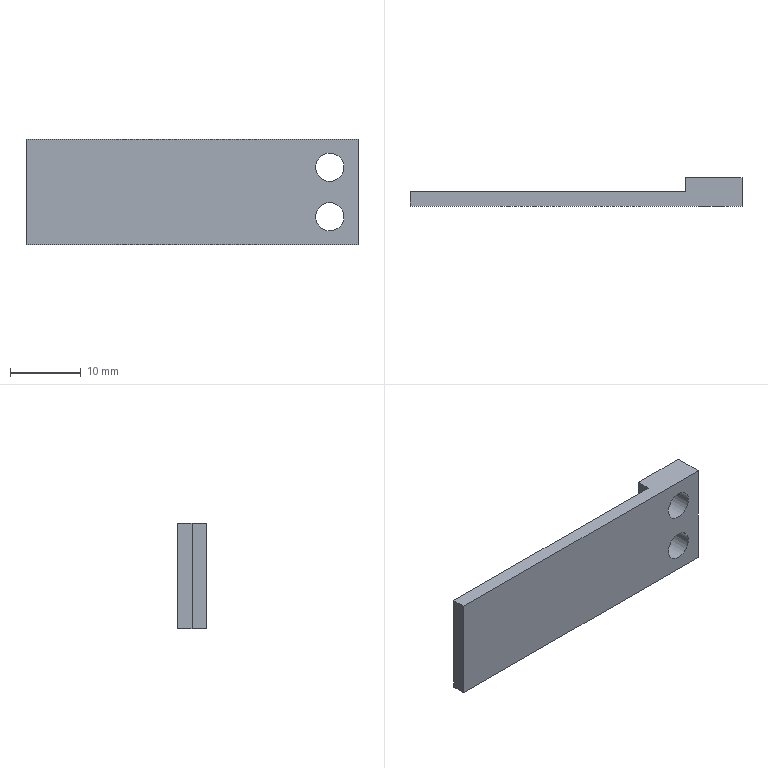Part | SolidWorks | features Extrusion 1, ICE 1 | 1 solid | 12 faces | box 47 x 4 x 15 mm | volume 1549 mm3 | plane 8 | cylinder 4 | commonest cylinder face diameters 4 x4
STEP:
#1=CARTESIAN_POINT('',(41.,0.,-3.5));
#2=VERTEX_POINT('',#1);
#3=CARTESIAN_POINT('',(45.,0.,-3.5));
#4=VERTEX_POINT('',#3);
#5=CARTESIAN_POINT('',(43.,0.,-3.5));
#6=DIRECTION('',(0.,-1.,0.));
#7=DIRECTION('',(0.,0.,1.));
#8=AXIS2_PLACEMENT_3D('',#5,#6,#7);
#9=CIRCLE('',#8,2.);
#10=EDGE_CURVE('',#2,#4,#9,.T.);
#11=ORIENTED_EDGE('',*,*,#10,.T.);
#12=CARTESIAN_POINT('',(45.,4.,-3.5));
#13=VERTEX_POINT('',#12);
#14=CARTESIAN_POINT('',(45.,-0.001,-3.5));
#15=DIRECTION('',(0.,1.,0.));
#16=VECTOR('',#15,1000.);
#17=LINE('',#14,#16);
#18=EDGE_CURVE('',#4,#13,#17,.T.);
#19=ORIENTED_EDGE('',*,*,#18,.T.);
#20=CARTESIAN_POINT('',(41.,4.,-3.5));
#21=VERTEX_POINT('',#20);
#22=CARTESIAN_POINT('',(43.,4.,-3.5));
#23=DIRECTION('',(0.,1.,0.));
#24=DIRECTION('',(-1.,0.,0.));
#25=AXIS2_PLACEMENT_3D('',#22,#23,#24);
#26=CIRCLE('',#25,2.);
#27=EDGE_CURVE('',#13,#21,#26,.T.);
#28=ORIENTED_EDGE('',*,*,#27,.T.);
#29=CARTESIAN_POINT('',(41.,-0.001,-3.5));
#30=DIRECTION('',(0.,1.,0.));
#31=VECTOR('',#30,1000.);
#32=LINE('',#29,#31);
#33=EDGE_CURVE('',#2,#21,#32,.T.);
#34=ORIENTED_EDGE('',*,*,#33,.F.);
#35=EDGE_LOOP('',(#11,#19,#28,#34));
#36=FACE_OUTER_BOUND('',#35,.T.);
#37=CARTESIAN_POINT('',(43.,-0.001,-3.5));
#38=DIRECTION('',(0.,1.,0.));
#39=DIRECTION('',(-1.,0.,0.));
#40=AXIS2_PLACEMENT_3D('',#37,#38,#39);
#41=CYLINDRICAL_SURFACE('',#40,2.);
#42=ADVANCED_FACE('',(#36),#41,.F.);
#43=CARTESIAN_POINT('',(41.,0.,3.5));
#44=VERTEX_POINT('',#43);
#45=CARTESIAN_POINT('',(45.,0.,3.5));
#46=VERTEX_POINT('',#45);
#47=CARTESIAN_POINT('',(43.,0.,3.5));
#48=DIRECTION('',(0.,-1.,0.));
#49=DIRECTION('',(0.,0.,1.));
#50=AXIS2_PLACEMENT_3D('',#47,#48,#49);
#51=CIRCLE('',#50,2.);
#52=EDGE_CURVE('',#44,#46,#51,.T.);
#53=ORIENTED_EDGE('',*,*,#52,.T.);
#54=CARTESIAN_POINT('',(45.,4.,3.5));
#55=VERTEX_POINT('',#54);
#56=CARTESIAN_POINT('',(45.,-0.001,3.5));
#57=DIRECTION('',(0.,1.,0.));
#58=VECTOR('',#57,1000.);
#59=LINE('',#56,#58);
#60=EDGE_CURVE('',#46,#55,#59,.T.);
#61=ORIENTED_EDGE('',*,*,#60,.T.);
#62=CARTESIAN_POINT('',(41.,4.,3.5));
#63=VERTEX_POINT('',#62);
#64=CARTESIAN_POINT('',(43.,4.,3.5));
#65=DIRECTION('',(0.,1.,0.));
#66=DIRECTION('',(-1.,0.,0.));
#67=AXIS2_PLACEMENT_3D('',#64,#65,#66);
#68=CIRCLE('',#67,2.);
#69=EDGE_CURVE('',#55,#63,#68,.T.);
#70=ORIENTED_EDGE('',*,*,#69,.T.);
#71=CARTESIAN_POINT('',(41.,-0.001,3.5));
#72=DIRECTION('',(0.,1.,0.));
#73=VECTOR('',#72,1000.);
#74=LINE('',#71,#73);
#75=EDGE_CURVE('',#44,#63,#74,.T.);
#76=ORIENTED_EDGE('',*,*,#75,.F.);
#77=EDGE_LOOP('',(#53,#61,#70,#76));
#78=FACE_OUTER_BOUND('',#77,.T.);
#79=CARTESIAN_POINT('',(43.,-0.001,3.5));
#80=DIRECTION('',(0.,1.,0.));
#81=DIRECTION('',(-1.,0.,0.));
#82=AXIS2_PLACEMENT_3D('',#79,#80,#81);
#83=CYLINDRICAL_SURFACE('',#82,2.);
#84=ADVANCED_FACE('',(#78),#83,.F.);
#85=CARTESIAN_POINT('',(0.,2.,-7.5));
#86=VERTEX_POINT('',#85);
#87=CARTESIAN_POINT('',(0.,0.,-7.5));
#88=VERTEX_POINT('',#87);
#89=CARTESIAN_POINT('',(0.,2.,-7.5));
#90=DIRECTION('',(0.,-1.,0.));
#91=VECTOR('',#90,1000.);
#92=LINE('',#89,#91);
#93=EDGE_CURVE('',#86,#88,#92,.T.);
#94=ORIENTED_EDGE('',*,*,#93,.T.);
#95=CARTESIAN_POINT('',(0.,0.,7.5));
#96=VERTEX_POINT('',#95);
#97=CARTESIAN_POINT('',(0.,0.,7.5));
#98=DIRECTION('',(0.,0.,-1.));
#99=VECTOR('',#98,1000.);
#100=LINE('',#97,#99);
#101=EDGE_CURVE('',#96,#88,#100,.T.);
#102=ORIENTED_EDGE('',*,*,#101,.F.);
#103=CARTESIAN_POINT('',(0.,2.,7.5));
#104=VERTEX_POINT('',#103);
#105=CARTESIAN_POINT('',(0.,2.,7.5));
#106=DIRECTION('',(0.,-1.,0.));
#107=VECTOR('',#106,1000.);
#108=LINE('',#105,#107);
#109=EDGE_CURVE('',#104,#96,#108,.T.);
#110=ORIENTED_EDGE('',*,*,#109,.F.);
#111=CARTESIAN_POINT('',(0.,2.,7.5));
#112=DIRECTION('',(0.,0.,-1.));
#113=VECTOR('',#112,1000.);
#114=LINE('',#111,#113);
#115=EDGE_CURVE('',#104,#86,#114,.T.);
#116=ORIENTED_EDGE('',*,*,#115,.T.);
#117=EDGE_LOOP('',(#94,#102,#110,#116));
#118=FACE_OUTER_BOUND('',#117,.T.);
#119=CARTESIAN_POINT('',(0.,2.,7.5));
#120=DIRECTION('',(1.,0.,0.));
#121=DIRECTION('',(0.,0.,-1.));
#122=AXIS2_PLACEMENT_3D('',#119,#120,#121);
#123=PLANE('',#122);
#124=ADVANCED_FACE('',(#118),#123,.F.);
#125=ORIENTED_EDGE('',*,*,#10,.F.);
#126=CARTESIAN_POINT('',(43.,0.,-3.5));
#127=DIRECTION('',(0.,-1.,0.));
#128=DIRECTION('',(0.,0.,1.));
#129=AXIS2_PLACEMENT_3D('',#126,#127,#128);
#130=CIRCLE('',#129,2.);
#131=EDGE_CURVE('',#4,#2,#130,.T.);
#132=ORIENTED_EDGE('',*,*,#131,.F.);
#133=EDGE_LOOP('',(#125,#132));
#134=FACE_BOUND('',#133,.T.);
#135=ORIENTED_EDGE('',*,*,#52,.F.);
#136=CARTESIAN_POINT('',(43.,0.,3.5));
#137=DIRECTION('',(0.,-1.,0.));
#138=DIRECTION('',(0.,0.,1.));
#139=AXIS2_PLACEMENT_3D('',#136,#137,#138);
#140=CIRCLE('',#139,2.);
#141=EDGE_CURVE('',#46,#44,#140,.T.);
#142=ORIENTED_EDGE('',*,*,#141,.F.);
#143=EDGE_LOOP('',(#135,#142));
#144=FACE_BOUND('',#143,.T.);
#145=CARTESIAN_POINT('',(47.,0.,-7.5));
#146=VERTEX_POINT('',#145);
#147=CARTESIAN_POINT('',(0.,0.,-7.5));
#148=DIRECTION('',(1.,0.,0.));
#149=VECTOR('',#148,1000.);
#150=LINE('',#147,#149);
#151=EDGE_CURVE('',#88,#146,#150,.T.);
#152=ORIENTED_EDGE('',*,*,#151,.T.);
#153=CARTESIAN_POINT('',(47.,0.,7.5));
#154=VERTEX_POINT('',#153);
#155=CARTESIAN_POINT('',(47.,0.,7.5));
#156=DIRECTION('',(0.,0.,-1.));
#157=VECTOR('',#156,1000.);
#158=LINE('',#155,#157);
#159=EDGE_CURVE('',#154,#146,#158,.T.);
#160=ORIENTED_EDGE('',*,*,#159,.F.);
#161=CARTESIAN_POINT('',(0.,0.,7.5));
#162=DIRECTION('',(1.,0.,0.));
#163=VECTOR('',#162,1000.);
#164=LINE('',#161,#163);
#165=EDGE_CURVE('',#96,#154,#164,.T.);
#166=ORIENTED_EDGE('',*,*,#165,.F.);
#167=ORIENTED_EDGE('',*,*,#101,.T.);
#168=EDGE_LOOP('',(#152,#160,#166,#167));
#169=FACE_OUTER_BOUND('',#168,.T.);
#170=CARTESIAN_POINT('',(0.,0.,7.5));
#171=DIRECTION('',(0.,1.,0.));
#172=DIRECTION('',(0.,0.,1.));
#173=AXIS2_PLACEMENT_3D('',#170,#171,#172);
#174=PLANE('',#173);
#175=ADVANCED_FACE('',(#134,#144,#169),#174,.F.);
#176=CARTESIAN_POINT('',(47.,4.,-7.5));
#177=VERTEX_POINT('',#176);
#178=CARTESIAN_POINT('',(47.,0.,-7.5));
#179=DIRECTION('',(0.,1.,0.));
#180=VECTOR('',#179,1000.);
#181=LINE('',#178,#180);
#182=EDGE_CURVE('',#146,#177,#181,.T.);
#183=ORIENTED_EDGE('',*,*,#182,.T.);
#184=CARTESIAN_POINT('',(47.,4.,7.5));
#185=VERTEX_POINT('',#184);
#186=CARTESIAN_POINT('',(47.,4.,7.5));
#187=DIRECTION('',(0.,0.,-1.));
#188=VECTOR('',#187,1000.);
#189=LINE('',#186,#188);
#190=EDGE_CURVE('',#185,#177,#189,.T.);
#191=ORIENTED_EDGE('',*,*,#190,.F.);
#192=CARTESIAN_POINT('',(47.,0.,7.5));
#193=DIRECTION('',(0.,1.,0.));
#194=VECTOR('',#193,1000.);
#195=LINE('',#192,#194);
#196=EDGE_CURVE('',#154,#185,#195,.T.);
#197=ORIENTED_EDGE('',*,*,#196,.F.);
#198=ORIENTED_EDGE('',*,*,#159,.T.);
#199=EDGE_LOOP('',(#183,#191,#197,#198));
#200=FACE_OUTER_BOUND('',#199,.T.);
#201=CARTESIAN_POINT('',(47.,0.,7.5));
#202=DIRECTION('',(-1.,0.,0.));
#203=DIRECTION('',(0.,0.,1.));
#204=AXIS2_PLACEMENT_3D('',#201,#202,#203);
#205=PLANE('',#204);
#206=ADVANCED_FACE('',(#200),#205,.F.);
#207=CARTESIAN_POINT('',(43.,4.,-3.5));
#208=DIRECTION('',(0.,1.,0.));
#209=DIRECTION('',(-1.,0.,0.));
#210=AXIS2_PLACEMENT_3D('',#207,#208,#209);
#211=CIRCLE('',#210,2.);
#212=EDGE_CURVE('',#21,#13,#211,.T.);
#213=ORIENTED_EDGE('',*,*,#212,.F.);
#214=ORIENTED_EDGE('',*,*,#27,.F.);
#215=EDGE_LOOP('',(#213,#214));
#216=FACE_BOUND('',#215,.T.);
#217=CARTESIAN_POINT('',(43.,4.,3.5));
#218=DIRECTION('',(0.,1.,0.));
#219=DIRECTION('',(-1.,0.,0.));
#220=AXIS2_PLACEMENT_3D('',#217,#218,#219);
#221=CIRCLE('',#220,2.);
#222=EDGE_CURVE('',#63,#55,#221,.T.);
#223=ORIENTED_EDGE('',*,*,#222,.F.);
#224=ORIENTED_EDGE('',*,*,#69,.F.);
#225=EDGE_LOOP('',(#223,#224));
#226=FACE_BOUND('',#225,.T.);
#227=CARTESIAN_POINT('',(39.,4.,-7.5));
#228=VERTEX_POINT('',#227);
#229=CARTESIAN_POINT('',(47.,4.,-7.5));
#230=DIRECTION('',(-1.,0.,0.));
#231=VECTOR('',#230,1000.);
#232=LINE('',#229,#231);
#233=EDGE_CURVE('',#177,#228,#232,.T.);
#234=ORIENTED_EDGE('',*,*,#233,.T.);
#235=CARTESIAN_POINT('',(39.,4.,7.5));
#236=VERTEX_POINT('',#235);
#237=CARTESIAN_POINT('',(39.,4.,7.5));
#238=DIRECTION('',(0.,0.,-1.));
#239=VECTOR('',#238,1000.);
#240=LINE('',#237,#239);
#241=EDGE_CURVE('',#236,#228,#240,.T.);
#242=ORIENTED_EDGE('',*,*,#241,.F.);
#243=CARTESIAN_POINT('',(47.,4.,7.5));
#244=DIRECTION('',(-1.,0.,0.));
#245=VECTOR('',#244,1000.);
#246=LINE('',#243,#245);
#247=EDGE_CURVE('',#185,#236,#246,.T.);
#248=ORIENTED_EDGE('',*,*,#247,.F.);
#249=ORIENTED_EDGE('',*,*,#190,.T.);
#250=EDGE_LOOP('',(#234,#242,#248,#249));
#251=FACE_OUTER_BOUND('',#250,.T.);
#252=CARTESIAN_POINT('',(47.,4.,7.5));
#253=DIRECTION('',(0.,-1.,0.));
#254=DIRECTION('',(1.,0.,0.));
#255=AXIS2_PLACEMENT_3D('',#252,#253,#254);
#256=PLANE('',#255);
#257=ADVANCED_FACE('',(#216,#226,#251),#256,.F.);
#258=CARTESIAN_POINT('',(39.,2.,-7.5));
#259=VERTEX_POINT('',#258);
#260=CARTESIAN_POINT('',(39.,4.,-7.5));
#261=DIRECTION('',(0.,-1.,0.));
#262=VECTOR('',#261,1000.);
#263=LINE('',#260,#262);
#264=EDGE_CURVE('',#228,#259,#263,.T.);
#265=ORIENTED_EDGE('',*,*,#264,.T.);
#266=CARTESIAN_POINT('',(39.,2.,7.5));
#267=VERTEX_POINT('',#266);
#268=CARTESIAN_POINT('',(39.,2.,7.5));
#269=DIRECTION('',(0.,0.,-1.));
#270=VECTOR('',#269,1000.);
#271=LINE('',#268,#270);
#272=EDGE_CURVE('',#267,#259,#271,.T.);
#273=ORIENTED_EDGE('',*,*,#272,.F.);
#274=CARTESIAN_POINT('',(39.,4.,7.5));
#275=DIRECTION('',(0.,-1.,0.));
#276=VECTOR('',#275,1000.);
#277=LINE('',#274,#276);
#278=EDGE_CURVE('',#236,#267,#277,.T.);
#279=ORIENTED_EDGE('',*,*,#278,.F.);
#280=ORIENTED_EDGE('',*,*,#241,.T.);
#281=EDGE_LOOP('',(#265,#273,#279,#280));
#282=FACE_OUTER_BOUND('',#281,.T.);
#283=CARTESIAN_POINT('',(39.,4.,7.5));
#284=DIRECTION('',(1.,0.,0.));
#285=DIRECTION('',(0.,0.,-1.));
#286=AXIS2_PLACEMENT_3D('',#283,#284,#285);
#287=PLANE('',#286);
#288=ADVANCED_FACE('',(#282),#287,.F.);
#289=CARTESIAN_POINT('',(39.,2.,-7.5));
#290=DIRECTION('',(-1.,0.,0.));
#291=VECTOR('',#290,1000.);
#292=LINE('',#289,#291);
#293=EDGE_CURVE('',#259,#86,#292,.T.);
#294=ORIENTED_EDGE('',*,*,#293,.T.);
#295=ORIENTED_EDGE('',*,*,#115,.F.);
#296=CARTESIAN_POINT('',(39.,2.,7.5));
#297=DIRECTION('',(-1.,0.,0.));
#298=VECTOR('',#297,1000.);
#299=LINE('',#296,#298);
#300=EDGE_CURVE('',#267,#104,#299,.T.);
#301=ORIENTED_EDGE('',*,*,#300,.F.);
#302=ORIENTED_EDGE('',*,*,#272,.T.);
#303=EDGE_LOOP('',(#294,#295,#301,#302));
#304=FACE_OUTER_BOUND('',#303,.T.);
#305=CARTESIAN_POINT('',(39.,2.,7.5));
#306=DIRECTION('',(0.,-1.,0.));
#307=DIRECTION('',(1.,0.,0.));
#308=AXIS2_PLACEMENT_3D('',#305,#306,#307);
#309=PLANE('',#308);
#310=ADVANCED_FACE('',(#304),#309,.F.);
#311=ORIENTED_EDGE('',*,*,#109,.T.);
#312=ORIENTED_EDGE('',*,*,#165,.T.);
#313=ORIENTED_EDGE('',*,*,#196,.T.);
#314=ORIENTED_EDGE('',*,*,#247,.T.);
#315=ORIENTED_EDGE('',*,*,#278,.T.);
#316=ORIENTED_EDGE('',*,*,#300,.T.);
#317=EDGE_LOOP('',(#311,#312,#313,#314,#315,#316));
#318=FACE_OUTER_BOUND('',#317,.T.);
#319=CARTESIAN_POINT('',(0.,0.,7.5));
#320=DIRECTION('',(0.,0.,1.));
#321=DIRECTION('',(1.,0.,0.));
#322=AXIS2_PLACEMENT_3D('',#319,#320,#321);
#323=PLANE('',#322);
#324=ADVANCED_FACE('',(#318),#323,.T.);
#325=ORIENTED_EDGE('',*,*,#93,.F.);
#326=ORIENTED_EDGE('',*,*,#293,.F.);
#327=ORIENTED_EDGE('',*,*,#264,.F.);
#328=ORIENTED_EDGE('',*,*,#233,.F.);
#329=ORIENTED_EDGE('',*,*,#182,.F.);
#330=ORIENTED_EDGE('',*,*,#151,.F.);
#331=EDGE_LOOP('',(#325,#326,#327,#328,#329,#330));
#332=FACE_OUTER_BOUND('',#331,.T.);
#333=CARTESIAN_POINT('',(0.,0.,-7.5));
#334=DIRECTION('',(0.,0.,1.));
#335=DIRECTION('',(1.,0.,0.));
#336=AXIS2_PLACEMENT_3D('',#333,#334,#335);
#337=PLANE('',#336);
#338=ADVANCED_FACE('',(#332),#337,.F.);
#339=ORIENTED_EDGE('',*,*,#60,.F.);
#340=ORIENTED_EDGE('',*,*,#141,.T.);
#341=ORIENTED_EDGE('',*,*,#75,.T.);
#342=ORIENTED_EDGE('',*,*,#222,.T.);
#343=EDGE_LOOP('',(#339,#340,#341,#342));
#344=FACE_OUTER_BOUND('',#343,.T.);
#345=CARTESIAN_POINT('',(43.,-0.001,3.5));
#346=DIRECTION('',(0.,1.,0.));
#347=DIRECTION('',(-1.,0.,0.));
#348=AXIS2_PLACEMENT_3D('',#345,#346,#347);
#349=CYLINDRICAL_SURFACE('',#348,2.);
#350=ADVANCED_FACE('',(#344),#349,.F.);
#351=ORIENTED_EDGE('',*,*,#18,.F.);
#352=ORIENTED_EDGE('',*,*,#131,.T.);
#353=ORIENTED_EDGE('',*,*,#33,.T.);
#354=ORIENTED_EDGE('',*,*,#212,.T.);
#355=EDGE_LOOP('',(#351,#352,#353,#354));
#356=FACE_OUTER_BOUND('',#355,.T.);
#357=CARTESIAN_POINT('',(43.,-0.001,-3.5));
#358=DIRECTION('',(0.,1.,0.));
#359=DIRECTION('',(-1.,0.,0.));
#360=AXIS2_PLACEMENT_3D('',#357,#358,#359);
#361=CYLINDRICAL_SURFACE('',#360,2.);
#362=ADVANCED_FACE('',(#356),#361,.F.);
#363=CLOSED_SHELL('',(#42,#84,#124,#175,#206,#257,#288,#310,#324,#338,#350,#362));
#364=MANIFOLD_SOLID_BREP('',#363);
#365=CARTESIAN_POINT('',(0.,0.,0.));
#366=DIRECTION('',(0.,0.,1.));
#367=DIRECTION('',(1.,0.,0.));
#368=AXIS2_PLACEMENT_3D('',#365,#366,#367);
#369=(LENGTH_UNIT()NAMED_UNIT(*)SI_UNIT(.MILLI.,.METRE.));
#370=UNCERTAINTY_MEASURE_WITH_UNIT(LENGTH_MEASURE(0.00001),#369,'','');
#371=(NAMED_UNIT(*)PLANE_ANGLE_UNIT()SI_UNIT($,.RADIAN.));
#372=(NAMED_UNIT(*)SI_UNIT($,.STERADIAN.)SOLID_ANGLE_UNIT());
#373=(GEOMETRIC_REPRESENTATION_CONTEXT(3)GLOBAL_UNCERTAINTY_ASSIGNED_CONTEXT((#370))GLOBAL_UNIT_ASSIGNED_CONTEXT((#369,#371,#372))REPRESENTATION_CONTEXT('',''));
#374=ADVANCED_BREP_SHAPE_REPRESENTATION('',(#364,#368),#373);